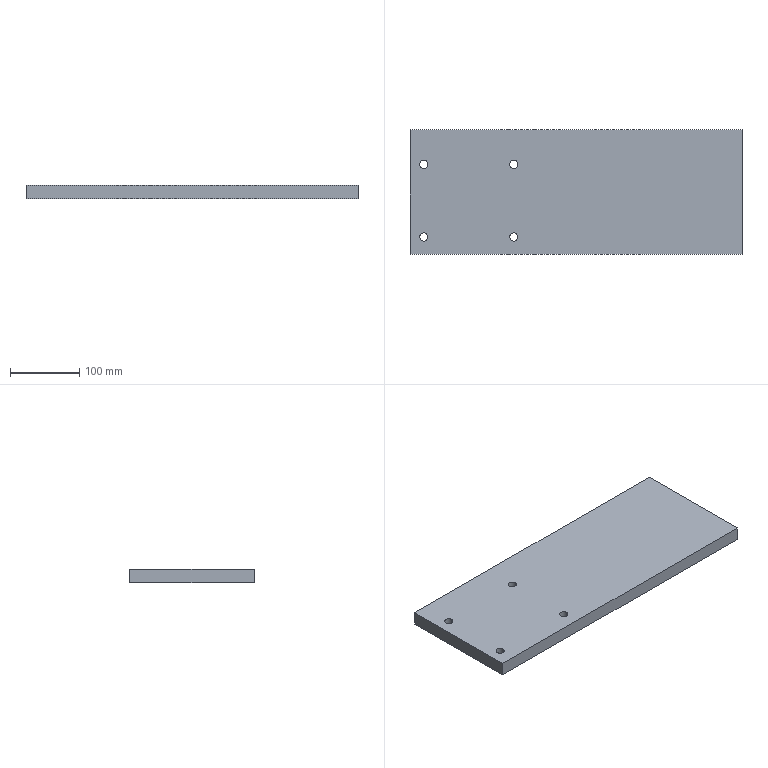Part | STEP file | Small Pad Plate | 1 solid | 14 faces | box 480 x 180 x 20 mm | volume 1718952 mm3 | cylinder 8 | plane 6 | commonest cylinder face diameters 12 x8
STEP:
#1=CARTESIAN_POINT('',(0.,0.,0.));
#2=DIRECTION('',(0.,0.,1.));
#3=DIRECTION('',(1.,0.,0.));
#4=AXIS2_PLACEMENT_3D('',#1,#2,#3);
#5=CARTESIAN_POINT('',(-84.,40.,0.));
#6=VERTEX_POINT('',#5);
#7=CARTESIAN_POINT('',(-84.,40.,20.));
#8=VERTEX_POINT('',#7);
#9=CARTESIAN_POINT('',(-84.,40.,20.));
#10=DIRECTION('',(0.,0.,1.));
#11=VECTOR('',#10,1.);
#12=LINE('',#9,#11);
#13=CARTESIAN_POINT('',(-90.,40.,20.));
#14=DIRECTION('',(0.,0.,1.));
#15=DIRECTION('',(1.,0.,0.));
#16=AXIS2_PLACEMENT_3D('',#13,#14,#15);
#17=CYLINDRICAL_SURFACE('',#16,6.);
#18=CARTESIAN_POINT('',(6.283,0.));
#19=DIRECTION('',(0.,1.));
#20=VECTOR('',#19,1.);
#21=LINE('',#18,#20);
#22=(GEOMETRIC_REPRESENTATION_CONTEXT(2)PARAMETRIC_REPRESENTATION_CONTEXT()REPRESENTATION_CONTEXT('',''));
#23=DEFINITIONAL_REPRESENTATION('',(#21),#22);
#24=PCURVE('',#17,#23);
#25=CARTESIAN_POINT('',(-90.,40.,20.));
#26=DIRECTION('',(0.,0.,1.));
#27=DIRECTION('',(1.,0.,0.));
#28=AXIS2_PLACEMENT_3D('',#25,#26,#27);
#29=CYLINDRICAL_SURFACE('',#28,6.);
#30=CARTESIAN_POINT('',(0.,0.));
#31=DIRECTION('',(0.,1.));
#32=VECTOR('',#31,1.);
#33=LINE('',#30,#32);
#34=(GEOMETRIC_REPRESENTATION_CONTEXT(2)PARAMETRIC_REPRESENTATION_CONTEXT()REPRESENTATION_CONTEXT('',''));
#35=DEFINITIONAL_REPRESENTATION('',(#33),#34);
#36=PCURVE('',#29,#35);
#37=SURFACE_CURVE('',#12,(#24,#36),.PCURVE_S1.);
#38=EDGE_CURVE('',#6,#8,#37,.T.);
#39=ORIENTED_EDGE('',*,*,#38,.T.);
#40=CARTESIAN_POINT('',(-96.,40.,20.));
#41=VERTEX_POINT('',#40);
#42=CARTESIAN_POINT('',(-90.,40.,20.));
#43=DIRECTION('',(0.,0.,1.));
#44=DIRECTION('',(1.,0.,0.));
#45=AXIS2_PLACEMENT_3D('',#42,#43,#44);
#46=CIRCLE('',#45,6.);
#47=CARTESIAN_POINT('',(0.,0.));
#48=DIRECTION('',(1.,0.));
#49=VECTOR('',#48,1.);
#50=LINE('',#47,#49);
#51=(GEOMETRIC_REPRESENTATION_CONTEXT(2)PARAMETRIC_REPRESENTATION_CONTEXT()REPRESENTATION_CONTEXT('',''));
#52=DEFINITIONAL_REPRESENTATION('',(#50),#51);
#53=PCURVE('',#17,#52);
#54=CARTESIAN_POINT('',(0.,0.,20.));
#55=DIRECTION('',(0.,0.,1.));
#56=DIRECTION('',(1.,0.,0.));
#57=AXIS2_PLACEMENT_3D('',#54,#55,#56);
#58=PLANE('',#57);
#59=CARTESIAN_POINT('',(-90.,40.));
#60=DIRECTION('',(1.,0.));
#61=AXIS2_PLACEMENT_2D('',#59,#60);
#62=CIRCLE('',#61,6.);
#63=(GEOMETRIC_REPRESENTATION_CONTEXT(2)PARAMETRIC_REPRESENTATION_CONTEXT()REPRESENTATION_CONTEXT('',''));
#64=DEFINITIONAL_REPRESENTATION('',(#62),#63);
#65=PCURVE('',#58,#64);
#66=SURFACE_CURVE('',#46,(#53,#65),.PCURVE_S1.);
#67=EDGE_CURVE('',#41,#8,#66,.T.);
#68=ORIENTED_EDGE('',*,*,#67,.F.);
#69=CARTESIAN_POINT('',(-96.,40.,0.));
#70=VERTEX_POINT('',#69);
#71=CARTESIAN_POINT('',(-96.,40.,20.));
#72=DIRECTION('',(0.,0.,1.));
#73=VECTOR('',#72,1.);
#74=LINE('',#71,#73);
#75=CARTESIAN_POINT('',(3.142,0.));
#76=DIRECTION('',(0.,1.));
#77=VECTOR('',#76,1.);
#78=LINE('',#75,#77);
#79=(GEOMETRIC_REPRESENTATION_CONTEXT(2)PARAMETRIC_REPRESENTATION_CONTEXT()REPRESENTATION_CONTEXT('',''));
#80=DEFINITIONAL_REPRESENTATION('',(#78),#79);
#81=PCURVE('',#17,#80);
#82=CARTESIAN_POINT('',(3.142,0.));
#83=DIRECTION('',(0.,1.));
#84=VECTOR('',#83,1.);
#85=LINE('',#82,#84);
#86=(GEOMETRIC_REPRESENTATION_CONTEXT(2)PARAMETRIC_REPRESENTATION_CONTEXT()REPRESENTATION_CONTEXT('',''));
#87=DEFINITIONAL_REPRESENTATION('',(#85),#86);
#88=PCURVE('',#29,#87);
#89=SURFACE_CURVE('',#74,(#81,#88),.PCURVE_S1.);
#90=EDGE_CURVE('',#70,#41,#89,.T.);
#91=ORIENTED_EDGE('',*,*,#90,.F.);
#92=CARTESIAN_POINT('',(-90.,40.,0.));
#93=DIRECTION('',(0.,0.,1.));
#94=DIRECTION('',(1.,0.,0.));
#95=AXIS2_PLACEMENT_3D('',#92,#93,#94);
#96=CIRCLE('',#95,6.);
#97=CARTESIAN_POINT('',(0.,-20.));
#98=DIRECTION('',(1.,0.));
#99=VECTOR('',#98,1.);
#100=LINE('',#97,#99);
#101=(GEOMETRIC_REPRESENTATION_CONTEXT(2)PARAMETRIC_REPRESENTATION_CONTEXT()REPRESENTATION_CONTEXT('',''));
#102=DEFINITIONAL_REPRESENTATION('',(#100),#101);
#103=PCURVE('',#17,#102);
#104=CARTESIAN_POINT('',(0.,0.,0.));
#105=DIRECTION('',(0.,0.,1.));
#106=DIRECTION('',(1.,0.,0.));
#107=AXIS2_PLACEMENT_3D('',#104,#105,#106);
#108=PLANE('',#107);
#109=CARTESIAN_POINT('',(-90.,40.));
#110=DIRECTION('',(1.,0.));
#111=AXIS2_PLACEMENT_2D('',#109,#110);
#112=CIRCLE('',#111,6.);
#113=(GEOMETRIC_REPRESENTATION_CONTEXT(2)PARAMETRIC_REPRESENTATION_CONTEXT()REPRESENTATION_CONTEXT('',''));
#114=DEFINITIONAL_REPRESENTATION('',(#112),#113);
#115=PCURVE('',#108,#114);
#116=SURFACE_CURVE('',#96,(#103,#115),.PCURVE_S1.);
#117=EDGE_CURVE('',#70,#6,#116,.T.);
#118=ORIENTED_EDGE('',*,*,#117,.T.);
#119=EDGE_LOOP('',(#39,#68,#91,#118));
#120=FACE_BOUND('',#119,.F.);
#121=ADVANCED_FACE('',(#120),#17,.F.);
#122=CARTESIAN_POINT('',(-84.,-65.,0.));
#123=VERTEX_POINT('',#122);
#124=CARTESIAN_POINT('',(-84.,-65.,20.));
#125=VERTEX_POINT('',#124);
#126=CARTESIAN_POINT('',(-84.,-65.,20.));
#127=DIRECTION('',(0.,0.,1.));
#128=VECTOR('',#127,1.);
#129=LINE('',#126,#128);
#130=CARTESIAN_POINT('',(-90.,-65.,20.));
#131=DIRECTION('',(0.,0.,1.));
#132=DIRECTION('',(1.,0.,0.));
#133=AXIS2_PLACEMENT_3D('',#130,#131,#132);
#134=CYLINDRICAL_SURFACE('',#133,6.);
#135=CARTESIAN_POINT('',(6.283,0.));
#136=DIRECTION('',(0.,1.));
#137=VECTOR('',#136,1.);
#138=LINE('',#135,#137);
#139=(GEOMETRIC_REPRESENTATION_CONTEXT(2)PARAMETRIC_REPRESENTATION_CONTEXT()REPRESENTATION_CONTEXT('',''));
#140=DEFINITIONAL_REPRESENTATION('',(#138),#139);
#141=PCURVE('',#134,#140);
#142=CARTESIAN_POINT('',(-90.,-65.,20.));
#143=DIRECTION('',(0.,0.,1.));
#144=DIRECTION('',(1.,0.,0.));
#145=AXIS2_PLACEMENT_3D('',#142,#143,#144);
#146=CYLINDRICAL_SURFACE('',#145,6.);
#147=CARTESIAN_POINT('',(0.,0.));
#148=DIRECTION('',(0.,1.));
#149=VECTOR('',#148,1.);
#150=LINE('',#147,#149);
#151=(GEOMETRIC_REPRESENTATION_CONTEXT(2)PARAMETRIC_REPRESENTATION_CONTEXT()REPRESENTATION_CONTEXT('',''));
#152=DEFINITIONAL_REPRESENTATION('',(#150),#151);
#153=PCURVE('',#146,#152);
#154=SURFACE_CURVE('',#129,(#141,#153),.PCURVE_S1.);
#155=EDGE_CURVE('',#123,#125,#154,.T.);
#156=ORIENTED_EDGE('',*,*,#155,.T.);
#157=CARTESIAN_POINT('',(-96.,-65.,20.));
#158=VERTEX_POINT('',#157);
#159=CARTESIAN_POINT('',(-90.,-65.,20.));
#160=DIRECTION('',(0.,0.,1.));
#161=DIRECTION('',(1.,0.,0.));
#162=AXIS2_PLACEMENT_3D('',#159,#160,#161);
#163=CIRCLE('',#162,6.);
#164=CARTESIAN_POINT('',(0.,0.));
#165=DIRECTION('',(1.,0.));
#166=VECTOR('',#165,1.);
#167=LINE('',#164,#166);
#168=(GEOMETRIC_REPRESENTATION_CONTEXT(2)PARAMETRIC_REPRESENTATION_CONTEXT()REPRESENTATION_CONTEXT('',''));
#169=DEFINITIONAL_REPRESENTATION('',(#167),#168);
#170=PCURVE('',#134,#169);
#171=CARTESIAN_POINT('',(-90.,-65.));
#172=DIRECTION('',(1.,0.));
#173=AXIS2_PLACEMENT_2D('',#171,#172);
#174=CIRCLE('',#173,6.);
#175=(GEOMETRIC_REPRESENTATION_CONTEXT(2)PARAMETRIC_REPRESENTATION_CONTEXT()REPRESENTATION_CONTEXT('',''));
#176=DEFINITIONAL_REPRESENTATION('',(#174),#175);
#177=PCURVE('',#58,#176);
#178=SURFACE_CURVE('',#163,(#170,#177),.PCURVE_S1.);
#179=EDGE_CURVE('',#158,#125,#178,.T.);
#180=ORIENTED_EDGE('',*,*,#179,.F.);
#181=CARTESIAN_POINT('',(-96.,-65.,0.));
#182=VERTEX_POINT('',#181);
#183=CARTESIAN_POINT('',(-96.,-65.,20.));
#184=DIRECTION('',(0.,0.,1.));
#185=VECTOR('',#184,1.);
#186=LINE('',#183,#185);
#187=CARTESIAN_POINT('',(3.142,0.));
#188=DIRECTION('',(0.,1.));
#189=VECTOR('',#188,1.);
#190=LINE('',#187,#189);
#191=(GEOMETRIC_REPRESENTATION_CONTEXT(2)PARAMETRIC_REPRESENTATION_CONTEXT()REPRESENTATION_CONTEXT('',''));
#192=DEFINITIONAL_REPRESENTATION('',(#190),#191);
#193=PCURVE('',#134,#192);
#194=CARTESIAN_POINT('',(3.142,0.));
#195=DIRECTION('',(0.,1.));
#196=VECTOR('',#195,1.);
#197=LINE('',#194,#196);
#198=(GEOMETRIC_REPRESENTATION_CONTEXT(2)PARAMETRIC_REPRESENTATION_CONTEXT()REPRESENTATION_CONTEXT('',''));
#199=DEFINITIONAL_REPRESENTATION('',(#197),#198);
#200=PCURVE('',#146,#199);
#201=SURFACE_CURVE('',#186,(#193,#200),.PCURVE_S1.);
#202=EDGE_CURVE('',#182,#158,#201,.T.);
#203=ORIENTED_EDGE('',*,*,#202,.F.);
#204=CARTESIAN_POINT('',(-90.,-65.,0.));
#205=DIRECTION('',(0.,0.,1.));
#206=DIRECTION('',(1.,0.,0.));
#207=AXIS2_PLACEMENT_3D('',#204,#205,#206);
#208=CIRCLE('',#207,6.);
#209=CARTESIAN_POINT('',(0.,-20.));
#210=DIRECTION('',(1.,0.));
#211=VECTOR('',#210,1.);
#212=LINE('',#209,#211);
#213=(GEOMETRIC_REPRESENTATION_CONTEXT(2)PARAMETRIC_REPRESENTATION_CONTEXT()REPRESENTATION_CONTEXT('',''));
#214=DEFINITIONAL_REPRESENTATION('',(#212),#213);
#215=PCURVE('',#134,#214);
#216=CARTESIAN_POINT('',(-90.,-65.));
#217=DIRECTION('',(1.,0.));
#218=AXIS2_PLACEMENT_2D('',#216,#217);
#219=CIRCLE('',#218,6.);
#220=(GEOMETRIC_REPRESENTATION_CONTEXT(2)PARAMETRIC_REPRESENTATION_CONTEXT()REPRESENTATION_CONTEXT('',''));
#221=DEFINITIONAL_REPRESENTATION('',(#219),#220);
#222=PCURVE('',#108,#221);
#223=SURFACE_CURVE('',#208,(#215,#222),.PCURVE_S1.);
#224=EDGE_CURVE('',#182,#123,#223,.T.);
#225=ORIENTED_EDGE('',*,*,#224,.T.);
#226=EDGE_LOOP('',(#156,#180,#203,#225));
#227=FACE_BOUND('',#226,.F.);
#228=ADVANCED_FACE('',(#227),#134,.F.);
#229=CARTESIAN_POINT('',(-214.,40.,0.));
#230=VERTEX_POINT('',#229);
#231=CARTESIAN_POINT('',(-214.,40.,20.));
#232=VERTEX_POINT('',#231);
#233=CARTESIAN_POINT('',(-214.,40.,20.));
#234=DIRECTION('',(0.,0.,1.));
#235=VECTOR('',#234,1.);
#236=LINE('',#233,#235);
#237=CARTESIAN_POINT('',(-220.,40.,20.));
#238=DIRECTION('',(0.,0.,1.));
#239=DIRECTION('',(1.,0.,0.));
#240=AXIS2_PLACEMENT_3D('',#237,#238,#239);
#241=CYLINDRICAL_SURFACE('',#240,6.);
#242=CARTESIAN_POINT('',(6.283,0.));
#243=DIRECTION('',(0.,1.));
#244=VECTOR('',#243,1.);
#245=LINE('',#242,#244);
#246=(GEOMETRIC_REPRESENTATION_CONTEXT(2)PARAMETRIC_REPRESENTATION_CONTEXT()REPRESENTATION_CONTEXT('',''));
#247=DEFINITIONAL_REPRESENTATION('',(#245),#246);
#248=PCURVE('',#241,#247);
#249=CARTESIAN_POINT('',(-220.,40.,20.));
#250=DIRECTION('',(0.,0.,1.));
#251=DIRECTION('',(1.,0.,0.));
#252=AXIS2_PLACEMENT_3D('',#249,#250,#251);
#253=CYLINDRICAL_SURFACE('',#252,6.);
#254=CARTESIAN_POINT('',(0.,0.));
#255=DIRECTION('',(0.,1.));
#256=VECTOR('',#255,1.);
#257=LINE('',#254,#256);
#258=(GEOMETRIC_REPRESENTATION_CONTEXT(2)PARAMETRIC_REPRESENTATION_CONTEXT()REPRESENTATION_CONTEXT('',''));
#259=DEFINITIONAL_REPRESENTATION('',(#257),#258);
#260=PCURVE('',#253,#259);
#261=SURFACE_CURVE('',#236,(#248,#260),.PCURVE_S1.);
#262=EDGE_CURVE('',#230,#232,#261,.T.);
#263=ORIENTED_EDGE('',*,*,#262,.T.);
#264=CARTESIAN_POINT('',(-226.,40.,20.));
#265=VERTEX_POINT('',#264);
#266=CARTESIAN_POINT('',(-220.,40.,20.));
#267=DIRECTION('',(0.,0.,1.));
#268=DIRECTION('',(1.,0.,0.));
#269=AXIS2_PLACEMENT_3D('',#266,#267,#268);
#270=CIRCLE('',#269,6.);
#271=CARTESIAN_POINT('',(0.,0.));
#272=DIRECTION('',(1.,0.));
#273=VECTOR('',#272,1.);
#274=LINE('',#271,#273);
#275=(GEOMETRIC_REPRESENTATION_CONTEXT(2)PARAMETRIC_REPRESENTATION_CONTEXT()REPRESENTATION_CONTEXT('',''));
#276=DEFINITIONAL_REPRESENTATION('',(#274),#275);
#277=PCURVE('',#241,#276);
#278=CARTESIAN_POINT('',(-220.,40.));
#279=DIRECTION('',(1.,0.));
#280=AXIS2_PLACEMENT_2D('',#278,#279);
#281=CIRCLE('',#280,6.);
#282=(GEOMETRIC_REPRESENTATION_CONTEXT(2)PARAMETRIC_REPRESENTATION_CONTEXT()REPRESENTATION_CONTEXT('',''));
#283=DEFINITIONAL_REPRESENTATION('',(#281),#282);
#284=PCURVE('',#58,#283);
#285=SURFACE_CURVE('',#270,(#277,#284),.PCURVE_S1.);
#286=EDGE_CURVE('',#265,#232,#285,.T.);
#287=ORIENTED_EDGE('',*,*,#286,.F.);
#288=CARTESIAN_POINT('',(-226.,40.,0.));
#289=VERTEX_POINT('',#288);
#290=CARTESIAN_POINT('',(-226.,40.,20.));
#291=DIRECTION('',(0.,0.,1.));
#292=VECTOR('',#291,1.);
#293=LINE('',#290,#292);
#294=CARTESIAN_POINT('',(3.142,0.));
#295=DIRECTION('',(0.,1.));
#296=VECTOR('',#295,1.);
#297=LINE('',#294,#296);
#298=(GEOMETRIC_REPRESENTATION_CONTEXT(2)PARAMETRIC_REPRESENTATION_CONTEXT()REPRESENTATION_CONTEXT('',''));
#299=DEFINITIONAL_REPRESENTATION('',(#297),#298);
#300=PCURVE('',#241,#299);
#301=CARTESIAN_POINT('',(3.142,0.));
#302=DIRECTION('',(0.,1.));
#303=VECTOR('',#302,1.);
#304=LINE('',#301,#303);
#305=(GEOMETRIC_REPRESENTATION_CONTEXT(2)PARAMETRIC_REPRESENTATION_CONTEXT()REPRESENTATION_CONTEXT('',''));
#306=DEFINITIONAL_REPRESENTATION('',(#304),#305);
#307=PCURVE('',#253,#306);
#308=SURFACE_CURVE('',#293,(#300,#307),.PCURVE_S1.);
#309=EDGE_CURVE('',#289,#265,#308,.T.);
#310=ORIENTED_EDGE('',*,*,#309,.F.);
#311=CARTESIAN_POINT('',(-220.,40.,0.));
#312=DIRECTION('',(0.,0.,1.));
#313=DIRECTION('',(1.,0.,0.));
#314=AXIS2_PLACEMENT_3D('',#311,#312,#313);
#315=CIRCLE('',#314,6.);
#316=CARTESIAN_POINT('',(0.,-20.));
#317=DIRECTION('',(1.,0.));
#318=VECTOR('',#317,1.);
#319=LINE('',#316,#318);
#320=(GEOMETRIC_REPRESENTATION_CONTEXT(2)PARAMETRIC_REPRESENTATION_CONTEXT()REPRESENTATION_CONTEXT('',''));
#321=DEFINITIONAL_REPRESENTATION('',(#319),#320);
#322=PCURVE('',#241,#321);
#323=CARTESIAN_POINT('',(-220.,40.));
#324=DIRECTION('',(1.,0.));
#325=AXIS2_PLACEMENT_2D('',#323,#324);
#326=CIRCLE('',#325,6.);
#327=(GEOMETRIC_REPRESENTATION_CONTEXT(2)PARAMETRIC_REPRESENTATION_CONTEXT()REPRESENTATION_CONTEXT('',''));
#328=DEFINITIONAL_REPRESENTATION('',(#326),#327);
#329=PCURVE('',#108,#328);
#330=SURFACE_CURVE('',#315,(#322,#329),.PCURVE_S1.);
#331=EDGE_CURVE('',#289,#230,#330,.T.);
#332=ORIENTED_EDGE('',*,*,#331,.T.);
#333=EDGE_LOOP('',(#263,#287,#310,#332));
#334=FACE_BOUND('',#333,.F.);
#335=ADVANCED_FACE('',(#334),#241,.F.);
#336=CARTESIAN_POINT('',(-214.,-65.,0.));
#337=VERTEX_POINT('',#336);
#338=CARTESIAN_POINT('',(-214.,-65.,20.));
#339=VERTEX_POINT('',#338);
#340=CARTESIAN_POINT('',(-214.,-65.,20.));
#341=DIRECTION('',(0.,0.,1.));
#342=VECTOR('',#341,1.);
#343=LINE('',#340,#342);
#344=CARTESIAN_POINT('',(-220.,-65.,20.));
#345=DIRECTION('',(0.,0.,1.));
#346=DIRECTION('',(1.,0.,0.));
#347=AXIS2_PLACEMENT_3D('',#344,#345,#346);
#348=CYLINDRICAL_SURFACE('',#347,6.);
#349=CARTESIAN_POINT('',(6.283,0.));
#350=DIRECTION('',(0.,1.));
#351=VECTOR('',#350,1.);
#352=LINE('',#349,#351);
#353=(GEOMETRIC_REPRESENTATION_CONTEXT(2)PARAMETRIC_REPRESENTATION_CONTEXT()REPRESENTATION_CONTEXT('',''));
#354=DEFINITIONAL_REPRESENTATION('',(#352),#353);
#355=PCURVE('',#348,#354);
#356=CARTESIAN_POINT('',(-220.,-65.,20.));
#357=DIRECTION('',(0.,0.,1.));
#358=DIRECTION('',(1.,0.,0.));
#359=AXIS2_PLACEMENT_3D('',#356,#357,#358);
#360=CYLINDRICAL_SURFACE('',#359,6.);
#361=CARTESIAN_POINT('',(0.,0.));
#362=DIRECTION('',(0.,1.));
#363=VECTOR('',#362,1.);
#364=LINE('',#361,#363);
#365=(GEOMETRIC_REPRESENTATION_CONTEXT(2)PARAMETRIC_REPRESENTATION_CONTEXT()REPRESENTATION_CONTEXT('',''));
#366=DEFINITIONAL_REPRESENTATION('',(#364),#365);
#367=PCURVE('',#360,#366);
#368=SURFACE_CURVE('',#343,(#355,#367),.PCURVE_S1.);
#369=EDGE_CURVE('',#337,#339,#368,.T.);
#370=ORIENTED_EDGE('',*,*,#369,.T.);
#371=CARTESIAN_POINT('',(-226.,-65.,20.));
#372=VERTEX_POINT('',#371);
#373=CARTESIAN_POINT('',(-220.,-65.,20.));
#374=DIRECTION('',(0.,0.,1.));
#375=DIRECTION('',(1.,0.,0.));
#376=AXIS2_PLACEMENT_3D('',#373,#374,#375);
#377=CIRCLE('',#376,6.);
#378=CARTESIAN_POINT('',(0.,0.));
#379=DIRECTION('',(1.,0.));
#380=VECTOR('',#379,1.);
#381=LINE('',#378,#380);
#382=(GEOMETRIC_REPRESENTATION_CONTEXT(2)PARAMETRIC_REPRESENTATION_CONTEXT()REPRESENTATION_CONTEXT('',''));
#383=DEFINITIONAL_REPRESENTATION('',(#381),#382);
#384=PCURVE('',#348,#383);
#385=CARTESIAN_POINT('',(-220.,-65.));
#386=DIRECTION('',(1.,0.));
#387=AXIS2_PLACEMENT_2D('',#385,#386);
#388=CIRCLE('',#387,6.);
#389=(GEOMETRIC_REPRESENTATION_CONTEXT(2)PARAMETRIC_REPRESENTATION_CONTEXT()REPRESENTATION_CONTEXT('',''));
#390=DEFINITIONAL_REPRESENTATION('',(#388),#389);
#391=PCURVE('',#58,#390);
#392=SURFACE_CURVE('',#377,(#384,#391),.PCURVE_S1.);
#393=EDGE_CURVE('',#372,#339,#392,.T.);
#394=ORIENTED_EDGE('',*,*,#393,.F.);
#395=CARTESIAN_POINT('',(-226.,-65.,0.));
#396=VERTEX_POINT('',#395);
#397=CARTESIAN_POINT('',(-226.,-65.,20.));
#398=DIRECTION('',(0.,0.,1.));
#399=VECTOR('',#398,1.);
#400=LINE('',#397,#399);
#401=CARTESIAN_POINT('',(3.142,0.));
#402=DIRECTION('',(0.,1.));
#403=VECTOR('',#402,1.);
#404=LINE('',#401,#403);
#405=(GEOMETRIC_REPRESENTATION_CONTEXT(2)PARAMETRIC_REPRESENTATION_CONTEXT()REPRESENTATION_CONTEXT('',''));
#406=DEFINITIONAL_REPRESENTATION('',(#404),#405);
#407=PCURVE('',#348,#406);
#408=CARTESIAN_POINT('',(3.142,0.));
#409=DIRECTION('',(0.,1.));
#410=VECTOR('',#409,1.);
#411=LINE('',#408,#410);
#412=(GEOMETRIC_REPRESENTATION_CONTEXT(2)PARAMETRIC_REPRESENTATION_CONTEXT()REPRESENTATION_CONTEXT('',''));
#413=DEFINITIONAL_REPRESENTATION('',(#411),#412);
#414=PCURVE('',#360,#413);
#415=SURFACE_CURVE('',#400,(#407,#414),.PCURVE_S1.);
#416=EDGE_CURVE('',#396,#372,#415,.T.);
#417=ORIENTED_EDGE('',*,*,#416,.F.);
#418=CARTESIAN_POINT('',(-220.,-65.,0.));
#419=DIRECTION('',(0.,0.,1.));
#420=DIRECTION('',(1.,0.,0.));
#421=AXIS2_PLACEMENT_3D('',#418,#419,#420);
#422=CIRCLE('',#421,6.);
#423=CARTESIAN_POINT('',(0.,-20.));
#424=DIRECTION('',(1.,0.));
#425=VECTOR('',#424,1.);
#426=LINE('',#423,#425);
#427=(GEOMETRIC_REPRESENTATION_CONTEXT(2)PARAMETRIC_REPRESENTATION_CONTEXT()REPRESENTATION_CONTEXT('',''));
#428=DEFINITIONAL_REPRESENTATION('',(#426),#427);
#429=PCURVE('',#348,#428);
#430=CARTESIAN_POINT('',(-220.,-65.));
#431=DIRECTION('',(1.,0.));
#432=AXIS2_PLACEMENT_2D('',#430,#431);
#433=CIRCLE('',#432,6.);
#434=(GEOMETRIC_REPRESENTATION_CONTEXT(2)PARAMETRIC_REPRESENTATION_CONTEXT()REPRESENTATION_CONTEXT('',''));
#435=DEFINITIONAL_REPRESENTATION('',(#433),#434);
#436=PCURVE('',#108,#435);
#437=SURFACE_CURVE('',#422,(#429,#436),.PCURVE_S1.);
#438=EDGE_CURVE('',#396,#337,#437,.T.);
#439=ORIENTED_EDGE('',*,*,#438,.T.);
#440=EDGE_LOOP('',(#370,#394,#417,#439));
#441=FACE_BOUND('',#440,.F.);
#442=ADVANCED_FACE('',(#441),#348,.F.);
#443=CARTESIAN_POINT('',(240.,-90.,0.));
#444=VERTEX_POINT('',#443);
#445=CARTESIAN_POINT('',(240.,90.,0.));
#446=VERTEX_POINT('',#445);
#447=CARTESIAN_POINT('',(240.,90.,0.));
#448=DIRECTION('',(0.,1.,0.));
#449=VECTOR('',#448,1.);
#450=LINE('',#447,#449);
#451=CARTESIAN_POINT('',(240.,90.,20.));
#452=DIRECTION('',(-1.,0.,0.));
#453=DIRECTION('',(0.,-1.,0.));
#454=AXIS2_PLACEMENT_3D('',#451,#452,#453);
#455=PLANE('',#454);
#456=CARTESIAN_POINT('',(0.,-20.));
#457=DIRECTION('',(-1.,0.));
#458=VECTOR('',#457,1.);
#459=LINE('',#456,#458);
#460=(GEOMETRIC_REPRESENTATION_CONTEXT(2)PARAMETRIC_REPRESENTATION_CONTEXT()REPRESENTATION_CONTEXT('',''));
#461=DEFINITIONAL_REPRESENTATION('',(#459),#460);
#462=PCURVE('',#455,#461);
#463=CARTESIAN_POINT('',(240.,90.));
#464=DIRECTION('',(0.,1.));
#465=VECTOR('',#464,1.);
#466=LINE('',#463,#465);
#467=(GEOMETRIC_REPRESENTATION_CONTEXT(2)PARAMETRIC_REPRESENTATION_CONTEXT()REPRESENTATION_CONTEXT('',''));
#468=DEFINITIONAL_REPRESENTATION('',(#466),#467);
#469=PCURVE('',#108,#468);
#470=SURFACE_CURVE('',#450,(#462,#469),.PCURVE_S1.);
#471=EDGE_CURVE('',#444,#446,#470,.T.);
#472=ORIENTED_EDGE('',*,*,#471,.T.);
#473=CARTESIAN_POINT('',(240.,90.,20.));
#474=VERTEX_POINT('',#473);
#475=CARTESIAN_POINT('',(240.,90.,20.));
#476=DIRECTION('',(0.,0.,-1.));
#477=VECTOR('',#476,1.);
#478=LINE('',#475,#477);
#479=CARTESIAN_POINT('',(0.,0.));
#480=DIRECTION('',(0.,-1.));
#481=VECTOR('',#480,1.);
#482=LINE('',#479,#481);
#483=(GEOMETRIC_REPRESENTATION_CONTEXT(2)PARAMETRIC_REPRESENTATION_CONTEXT()REPRESENTATION_CONTEXT('',''));
#484=DEFINITIONAL_REPRESENTATION('',(#482),#483);
#485=PCURVE('',#455,#484);
#486=CARTESIAN_POINT('',(-240.,90.,20.));
#487=DIRECTION('',(0.,-1.,0.));
#488=DIRECTION('',(0.,0.,-1.));
#489=AXIS2_PLACEMENT_3D('',#486,#487,#488);
#490=PLANE('',#489);
#491=CARTESIAN_POINT('',(0.,480.));
#492=DIRECTION('',(1.,0.));
#493=VECTOR('',#492,1.);
#494=LINE('',#491,#493);
#495=(GEOMETRIC_REPRESENTATION_CONTEXT(2)PARAMETRIC_REPRESENTATION_CONTEXT()REPRESENTATION_CONTEXT('',''));
#496=DEFINITIONAL_REPRESENTATION('',(#494),#495);
#497=PCURVE('',#490,#496);
#498=SURFACE_CURVE('',#478,(#485,#497),.PCURVE_S1.);
#499=EDGE_CURVE('',#474,#446,#498,.T.);
#500=ORIENTED_EDGE('',*,*,#499,.F.);
#501=CARTESIAN_POINT('',(240.,-90.,20.));
#502=VERTEX_POINT('',#501);
#503=CARTESIAN_POINT('',(240.,90.,20.));
#504=DIRECTION('',(0.,1.,0.));
#505=VECTOR('',#504,1.);
#506=LINE('',#503,#505);
#507=CARTESIAN_POINT('',(0.,0.));
#508=DIRECTION('',(-1.,0.));
#509=VECTOR('',#508,1.);
#510=LINE('',#507,#509);
#511=(GEOMETRIC_REPRESENTATION_CONTEXT(2)PARAMETRIC_REPRESENTATION_CONTEXT()REPRESENTATION_CONTEXT('',''));
#512=DEFINITIONAL_REPRESENTATION('',(#510),#511);
#513=PCURVE('',#455,#512);
#514=CARTESIAN_POINT('',(240.,90.));
#515=DIRECTION('',(0.,1.));
#516=VECTOR('',#515,1.);
#517=LINE('',#514,#516);
#518=(GEOMETRIC_REPRESENTATION_CONTEXT(2)PARAMETRIC_REPRESENTATION_CONTEXT()REPRESENTATION_CONTEXT('',''));
#519=DEFINITIONAL_REPRESENTATION('',(#517),#518);
#520=PCURVE('',#58,#519);
#521=SURFACE_CURVE('',#506,(#513,#520),.PCURVE_S1.);
#522=EDGE_CURVE('',#502,#474,#521,.T.);
#523=ORIENTED_EDGE('',*,*,#522,.F.);
#524=CARTESIAN_POINT('',(240.,-90.,20.));
#525=DIRECTION('',(0.,0.,-1.));
#526=VECTOR('',#525,1.);
#527=LINE('',#524,#526);
#528=CARTESIAN_POINT('',(180.,0.));
#529=DIRECTION('',(0.,-1.));
#530=VECTOR('',#529,1.);
#531=LINE('',#528,#530);
#532=(GEOMETRIC_REPRESENTATION_CONTEXT(2)PARAMETRIC_REPRESENTATION_CONTEXT()REPRESENTATION_CONTEXT('',''));
#533=DEFINITIONAL_REPRESENTATION('',(#531),#532);
#534=PCURVE('',#455,#533);
#535=CARTESIAN_POINT('',(-240.,-90.,20.));
#536=DIRECTION('',(0.,1.,0.));
#537=DIRECTION('',(0.,0.,1.));
#538=AXIS2_PLACEMENT_3D('',#535,#536,#537);
#539=PLANE('',#538);
#540=CARTESIAN_POINT('',(0.,480.));
#541=DIRECTION('',(-1.,0.));
#542=VECTOR('',#541,1.);
#543=LINE('',#540,#542);
#544=(GEOMETRIC_REPRESENTATION_CONTEXT(2)PARAMETRIC_REPRESENTATION_CONTEXT()REPRESENTATION_CONTEXT('',''));
#545=DEFINITIONAL_REPRESENTATION('',(#543),#544);
#546=PCURVE('',#539,#545);
#547=SURFACE_CURVE('',#527,(#534,#546),.PCURVE_S1.);
#548=EDGE_CURVE('',#502,#444,#547,.T.);
#549=ORIENTED_EDGE('',*,*,#548,.T.);
#550=EDGE_LOOP('',(#472,#500,#523,#549));
#551=FACE_BOUND('',#550,.T.);
#552=ADVANCED_FACE('',(#551),#455,.F.);
#553=CARTESIAN_POINT('',(-240.,90.,0.));
#554=VERTEX_POINT('',#553);
#555=CARTESIAN_POINT('',(-240.,90.,0.));
#556=DIRECTION('',(-1.,0.,0.));
#557=VECTOR('',#556,1.);
#558=LINE('',#555,#557);
#559=CARTESIAN_POINT('',(20.,0.));
#560=DIRECTION('',(0.,-1.));
#561=VECTOR('',#560,1.);
#562=LINE('',#559,#561);
#563=(GEOMETRIC_REPRESENTATION_CONTEXT(2)PARAMETRIC_REPRESENTATION_CONTEXT()REPRESENTATION_CONTEXT('',''));
#564=DEFINITIONAL_REPRESENTATION('',(#562),#563);
#565=PCURVE('',#490,#564);
#566=CARTESIAN_POINT('',(-240.,90.));
#567=DIRECTION('',(-1.,0.));
#568=VECTOR('',#567,1.);
#569=LINE('',#566,#568);
#570=(GEOMETRIC_REPRESENTATION_CONTEXT(2)PARAMETRIC_REPRESENTATION_CONTEXT()REPRESENTATION_CONTEXT('',''));
#571=DEFINITIONAL_REPRESENTATION('',(#569),#570);
#572=PCURVE('',#108,#571);
#573=SURFACE_CURVE('',#558,(#565,#572),.PCURVE_S1.);
#574=EDGE_CURVE('',#446,#554,#573,.T.);
#575=ORIENTED_EDGE('',*,*,#574,.T.);
#576=CARTESIAN_POINT('',(-240.,90.,20.));
#577=VERTEX_POINT('',#576);
#578=CARTESIAN_POINT('',(-240.,90.,20.));
#579=DIRECTION('',(0.,0.,-1.));
#580=VECTOR('',#579,1.);
#581=LINE('',#578,#580);
#582=CARTESIAN_POINT('',(0.,0.));
#583=DIRECTION('',(1.,0.));
#584=VECTOR('',#583,1.);
#585=LINE('',#582,#584);
#586=(GEOMETRIC_REPRESENTATION_CONTEXT(2)PARAMETRIC_REPRESENTATION_CONTEXT()REPRESENTATION_CONTEXT('',''));
#587=DEFINITIONAL_REPRESENTATION('',(#585),#586);
#588=PCURVE('',#490,#587);
#589=CARTESIAN_POINT('',(-240.,90.,20.));
#590=DIRECTION('',(1.,0.,0.));
#591=DIRECTION('',(0.,1.,0.));
#592=AXIS2_PLACEMENT_3D('',#589,#590,#591);
#593=PLANE('',#592);
#594=CARTESIAN_POINT('',(0.,0.));
#595=DIRECTION('',(0.,-1.));
#596=VECTOR('',#595,1.);
#597=LINE('',#594,#596);
#598=(GEOMETRIC_REPRESENTATION_CONTEXT(2)PARAMETRIC_REPRESENTATION_CONTEXT()REPRESENTATION_CONTEXT('',''));
#599=DEFINITIONAL_REPRESENTATION('',(#597),#598);
#600=PCURVE('',#593,#599);
#601=SURFACE_CURVE('',#581,(#588,#600),.PCURVE_S1.);
#602=EDGE_CURVE('',#577,#554,#601,.T.);
#603=ORIENTED_EDGE('',*,*,#602,.F.);
#604=CARTESIAN_POINT('',(-240.,90.,20.));
#605=DIRECTION('',(-1.,0.,0.));
#606=VECTOR('',#605,1.);
#607=LINE('',#604,#606);
#608=CARTESIAN_POINT('',(0.,0.));
#609=DIRECTION('',(0.,-1.));
#610=VECTOR('',#609,1.);
#611=LINE('',#608,#610);
#612=(GEOMETRIC_REPRESENTATION_CONTEXT(2)PARAMETRIC_REPRESENTATION_CONTEXT()REPRESENTATION_CONTEXT('',''));
#613=DEFINITIONAL_REPRESENTATION('',(#611),#612);
#614=PCURVE('',#490,#613);
#615=CARTESIAN_POINT('',(-240.,90.));
#616=DIRECTION('',(-1.,0.));
#617=VECTOR('',#616,1.);
#618=LINE('',#615,#617);
#619=(GEOMETRIC_REPRESENTATION_CONTEXT(2)PARAMETRIC_REPRESENTATION_CONTEXT()REPRESENTATION_CONTEXT('',''));
#620=DEFINITIONAL_REPRESENTATION('',(#618),#619);
#621=PCURVE('',#58,#620);
#622=SURFACE_CURVE('',#607,(#614,#621),.PCURVE_S1.);
#623=EDGE_CURVE('',#474,#577,#622,.T.);
#624=ORIENTED_EDGE('',*,*,#623,.F.);
#625=ORIENTED_EDGE('',*,*,#499,.T.);
#626=EDGE_LOOP('',(#575,#603,#624,#625));
#627=FACE_BOUND('',#626,.T.);
#628=ADVANCED_FACE('',(#627),#490,.F.);
#629=CARTESIAN_POINT('',(-240.,-90.,0.));
#630=VERTEX_POINT('',#629);
#631=CARTESIAN_POINT('',(-240.,90.,0.));
#632=DIRECTION('',(0.,-1.,0.));
#633=VECTOR('',#632,1.);
#634=LINE('',#631,#633);
#635=CARTESIAN_POINT('',(0.,-20.));
#636=DIRECTION('',(-1.,0.));
#637=VECTOR('',#636,1.);
#638=LINE('',#635,#637);
#639=(GEOMETRIC_REPRESENTATION_CONTEXT(2)PARAMETRIC_REPRESENTATION_CONTEXT()REPRESENTATION_CONTEXT('',''));
#640=DEFINITIONAL_REPRESENTATION('',(#638),#639);
#641=PCURVE('',#593,#640);
#642=CARTESIAN_POINT('',(-240.,90.));
#643=DIRECTION('',(0.,-1.));
#644=VECTOR('',#643,1.);
#645=LINE('',#642,#644);
#646=(GEOMETRIC_REPRESENTATION_CONTEXT(2)PARAMETRIC_REPRESENTATION_CONTEXT()REPRESENTATION_CONTEXT('',''));
#647=DEFINITIONAL_REPRESENTATION('',(#645),#646);
#648=PCURVE('',#108,#647);
#649=SURFACE_CURVE('',#634,(#641,#648),.PCURVE_S1.);
#650=EDGE_CURVE('',#554,#630,#649,.T.);
#651=ORIENTED_EDGE('',*,*,#650,.T.);
#652=CARTESIAN_POINT('',(-240.,-90.,20.));
#653=VERTEX_POINT('',#652);
#654=CARTESIAN_POINT('',(-240.,-90.,20.));
#655=DIRECTION('',(0.,0.,-1.));
#656=VECTOR('',#655,1.);
#657=LINE('',#654,#656);
#658=CARTESIAN_POINT('',(-180.,0.));
#659=DIRECTION('',(0.,-1.));
#660=VECTOR('',#659,1.);
#661=LINE('',#658,#660);
#662=(GEOMETRIC_REPRESENTATION_CONTEXT(2)PARAMETRIC_REPRESENTATION_CONTEXT()REPRESENTATION_CONTEXT('',''));
#663=DEFINITIONAL_REPRESENTATION('',(#661),#662);
#664=PCURVE('',#593,#663);
#665=CARTESIAN_POINT('',(0.,0.));
#666=DIRECTION('',(-1.,0.));
#667=VECTOR('',#666,1.);
#668=LINE('',#665,#667);
#669=(GEOMETRIC_REPRESENTATION_CONTEXT(2)PARAMETRIC_REPRESENTATION_CONTEXT()REPRESENTATION_CONTEXT('',''));
#670=DEFINITIONAL_REPRESENTATION('',(#668),#669);
#671=PCURVE('',#539,#670);
#672=SURFACE_CURVE('',#657,(#664,#671),.PCURVE_S1.);
#673=EDGE_CURVE('',#653,#630,#672,.T.);
#674=ORIENTED_EDGE('',*,*,#673,.F.);
#675=CARTESIAN_POINT('',(-240.,90.,20.));
#676=DIRECTION('',(0.,-1.,0.));
#677=VECTOR('',#676,1.);
#678=LINE('',#675,#677);
#679=CARTESIAN_POINT('',(0.,0.));
#680=DIRECTION('',(-1.,0.));
#681=VECTOR('',#680,1.);
#682=LINE('',#679,#681);
#683=(GEOMETRIC_REPRESENTATION_CONTEXT(2)PARAMETRIC_REPRESENTATION_CONTEXT()REPRESENTATION_CONTEXT('',''));
#684=DEFINITIONAL_REPRESENTATION('',(#682),#683);
#685=PCURVE('',#593,#684);
#686=CARTESIAN_POINT('',(-240.,90.));
#687=DIRECTION('',(0.,-1.));
#688=VECTOR('',#687,1.);
#689=LINE('',#686,#688);
#690=(GEOMETRIC_REPRESENTATION_CONTEXT(2)PARAMETRIC_REPRESENTATION_CONTEXT()REPRESENTATION_CONTEXT('',''));
#691=DEFINITIONAL_REPRESENTATION('',(#689),#690);
#692=PCURVE('',#58,#691);
#693=SURFACE_CURVE('',#678,(#685,#692),.PCURVE_S1.);
#694=EDGE_CURVE('',#577,#653,#693,.T.);
#695=ORIENTED_EDGE('',*,*,#694,.F.);
#696=ORIENTED_EDGE('',*,*,#602,.T.);
#697=EDGE_LOOP('',(#651,#674,#695,#696));
#698=FACE_BOUND('',#697,.T.);
#699=ADVANCED_FACE('',(#698),#593,.F.);
#700=CARTESIAN_POINT('',(-240.,-90.,0.));
#701=DIRECTION('',(1.,0.,0.));
#702=VECTOR('',#701,1.);
#703=LINE('',#700,#702);
#704=CARTESIAN_POINT('',(-20.,0.));
#705=DIRECTION('',(0.,1.));
#706=VECTOR('',#705,1.);
#707=LINE('',#704,#706);
#708=(GEOMETRIC_REPRESENTATION_CONTEXT(2)PARAMETRIC_REPRESENTATION_CONTEXT()REPRESENTATION_CONTEXT('',''));
#709=DEFINITIONAL_REPRESENTATION('',(#707),#708);
#710=PCURVE('',#539,#709);
#711=CARTESIAN_POINT('',(-240.,-90.));
#712=DIRECTION('',(1.,0.));
#713=VECTOR('',#712,1.);
#714=LINE('',#711,#713);
#715=(GEOMETRIC_REPRESENTATION_CONTEXT(2)PARAMETRIC_REPRESENTATION_CONTEXT()REPRESENTATION_CONTEXT('',''));
#716=DEFINITIONAL_REPRESENTATION('',(#714),#715);
#717=PCURVE('',#108,#716);
#718=SURFACE_CURVE('',#703,(#710,#717),.PCURVE_S1.);
#719=EDGE_CURVE('',#630,#444,#718,.T.);
#720=ORIENTED_EDGE('',*,*,#719,.T.);
#721=ORIENTED_EDGE('',*,*,#548,.F.);
#722=CARTESIAN_POINT('',(-240.,-90.,20.));
#723=DIRECTION('',(1.,0.,0.));
#724=VECTOR('',#723,1.);
#725=LINE('',#722,#724);
#726=CARTESIAN_POINT('',(0.,0.));
#727=DIRECTION('',(0.,1.));
#728=VECTOR('',#727,1.);
#729=LINE('',#726,#728);
#730=(GEOMETRIC_REPRESENTATION_CONTEXT(2)PARAMETRIC_REPRESENTATION_CONTEXT()REPRESENTATION_CONTEXT('',''));
#731=DEFINITIONAL_REPRESENTATION('',(#729),#730);
#732=PCURVE('',#539,#731);
#733=CARTESIAN_POINT('',(-240.,-90.));
#734=DIRECTION('',(1.,0.));
#735=VECTOR('',#734,1.);
#736=LINE('',#733,#735);
#737=(GEOMETRIC_REPRESENTATION_CONTEXT(2)PARAMETRIC_REPRESENTATION_CONTEXT()REPRESENTATION_CONTEXT('',''));
#738=DEFINITIONAL_REPRESENTATION('',(#736),#737);
#739=PCURVE('',#58,#738);
#740=SURFACE_CURVE('',#725,(#732,#739),.PCURVE_S1.);
#741=EDGE_CURVE('',#653,#502,#740,.T.);
#742=ORIENTED_EDGE('',*,*,#741,.F.);
#743=ORIENTED_EDGE('',*,*,#673,.T.);
#744=EDGE_LOOP('',(#720,#721,#742,#743));
#745=FACE_BOUND('',#744,.T.);
#746=ADVANCED_FACE('',(#745),#539,.F.);
#747=CARTESIAN_POINT('',(-90.,40.,20.));
#748=DIRECTION('',(0.,0.,1.));
#749=DIRECTION('',(1.,0.,0.));
#750=AXIS2_PLACEMENT_3D('',#747,#748,#749);
#751=CIRCLE('',#750,6.);
#752=CARTESIAN_POINT('',(-90.,40.));
#753=DIRECTION('',(1.,0.));
#754=AXIS2_PLACEMENT_2D('',#752,#753);
#755=CIRCLE('',#754,6.);
#756=(GEOMETRIC_REPRESENTATION_CONTEXT(2)PARAMETRIC_REPRESENTATION_CONTEXT()REPRESENTATION_CONTEXT('',''));
#757=DEFINITIONAL_REPRESENTATION('',(#755),#756);
#758=PCURVE('',#58,#757);
#759=CARTESIAN_POINT('',(0.,0.));
#760=DIRECTION('',(1.,0.));
#761=VECTOR('',#760,1.);
#762=LINE('',#759,#761);
#763=(GEOMETRIC_REPRESENTATION_CONTEXT(2)PARAMETRIC_REPRESENTATION_CONTEXT()REPRESENTATION_CONTEXT('',''));
#764=DEFINITIONAL_REPRESENTATION('',(#762),#763);
#765=PCURVE('',#29,#764);
#766=SURFACE_CURVE('',#751,(#758,#765),.PCURVE_S1.);
#767=EDGE_CURVE('',#8,#41,#766,.T.);
#768=ORIENTED_EDGE('',*,*,#767,.F.);
#769=ORIENTED_EDGE('',*,*,#67,.F.);
#770=EDGE_LOOP('',(#768,#769));
#771=FACE_BOUND('',#770,.T.);
#772=CARTESIAN_POINT('',(-90.,-65.,20.));
#773=DIRECTION('',(0.,0.,1.));
#774=DIRECTION('',(1.,0.,0.));
#775=AXIS2_PLACEMENT_3D('',#772,#773,#774);
#776=CIRCLE('',#775,6.);
#777=CARTESIAN_POINT('',(-90.,-65.));
#778=DIRECTION('',(1.,0.));
#779=AXIS2_PLACEMENT_2D('',#777,#778);
#780=CIRCLE('',#779,6.);
#781=(GEOMETRIC_REPRESENTATION_CONTEXT(2)PARAMETRIC_REPRESENTATION_CONTEXT()REPRESENTATION_CONTEXT('',''));
#782=DEFINITIONAL_REPRESENTATION('',(#780),#781);
#783=PCURVE('',#58,#782);
#784=CARTESIAN_POINT('',(0.,0.));
#785=DIRECTION('',(1.,0.));
#786=VECTOR('',#785,1.);
#787=LINE('',#784,#786);
#788=(GEOMETRIC_REPRESENTATION_CONTEXT(2)PARAMETRIC_REPRESENTATION_CONTEXT()REPRESENTATION_CONTEXT('',''));
#789=DEFINITIONAL_REPRESENTATION('',(#787),#788);
#790=PCURVE('',#146,#789);
#791=SURFACE_CURVE('',#776,(#783,#790),.PCURVE_S1.);
#792=EDGE_CURVE('',#125,#158,#791,.T.);
#793=ORIENTED_EDGE('',*,*,#792,.F.);
#794=ORIENTED_EDGE('',*,*,#179,.F.);
#795=EDGE_LOOP('',(#793,#794));
#796=FACE_BOUND('',#795,.T.);
#797=CARTESIAN_POINT('',(-220.,40.,20.));
#798=DIRECTION('',(0.,0.,1.));
#799=DIRECTION('',(1.,0.,0.));
#800=AXIS2_PLACEMENT_3D('',#797,#798,#799);
#801=CIRCLE('',#800,6.);
#802=CARTESIAN_POINT('',(-220.,40.));
#803=DIRECTION('',(1.,0.));
#804=AXIS2_PLACEMENT_2D('',#802,#803);
#805=CIRCLE('',#804,6.);
#806=(GEOMETRIC_REPRESENTATION_CONTEXT(2)PARAMETRIC_REPRESENTATION_CONTEXT()REPRESENTATION_CONTEXT('',''));
#807=DEFINITIONAL_REPRESENTATION('',(#805),#806);
#808=PCURVE('',#58,#807);
#809=CARTESIAN_POINT('',(0.,0.));
#810=DIRECTION('',(1.,0.));
#811=VECTOR('',#810,1.);
#812=LINE('',#809,#811);
#813=(GEOMETRIC_REPRESENTATION_CONTEXT(2)PARAMETRIC_REPRESENTATION_CONTEXT()REPRESENTATION_CONTEXT('',''));
#814=DEFINITIONAL_REPRESENTATION('',(#812),#813);
#815=PCURVE('',#253,#814);
#816=SURFACE_CURVE('',#801,(#808,#815),.PCURVE_S1.);
#817=EDGE_CURVE('',#232,#265,#816,.T.);
#818=ORIENTED_EDGE('',*,*,#817,.F.);
#819=ORIENTED_EDGE('',*,*,#286,.F.);
#820=EDGE_LOOP('',(#818,#819));
#821=FACE_BOUND('',#820,.T.);
#822=CARTESIAN_POINT('',(-220.,-65.,20.));
#823=DIRECTION('',(0.,0.,1.));
#824=DIRECTION('',(1.,0.,0.));
#825=AXIS2_PLACEMENT_3D('',#822,#823,#824);
#826=CIRCLE('',#825,6.);
#827=CARTESIAN_POINT('',(-220.,-65.));
#828=DIRECTION('',(1.,0.));
#829=AXIS2_PLACEMENT_2D('',#827,#828);
#830=CIRCLE('',#829,6.);
#831=(GEOMETRIC_REPRESENTATION_CONTEXT(2)PARAMETRIC_REPRESENTATION_CONTEXT()REPRESENTATION_CONTEXT('',''));
#832=DEFINITIONAL_REPRESENTATION('',(#830),#831);
#833=PCURVE('',#58,#832);
#834=CARTESIAN_POINT('',(0.,0.));
#835=DIRECTION('',(1.,0.));
#836=VECTOR('',#835,1.);
#837=LINE('',#834,#836);
#838=(GEOMETRIC_REPRESENTATION_CONTEXT(2)PARAMETRIC_REPRESENTATION_CONTEXT()REPRESENTATION_CONTEXT('',''));
#839=DEFINITIONAL_REPRESENTATION('',(#837),#838);
#840=PCURVE('',#360,#839);
#841=SURFACE_CURVE('',#826,(#833,#840),.PCURVE_S1.);
#842=EDGE_CURVE('',#339,#372,#841,.T.);
#843=ORIENTED_EDGE('',*,*,#842,.F.);
#844=ORIENTED_EDGE('',*,*,#393,.F.);
#845=EDGE_LOOP('',(#843,#844));
#846=FACE_BOUND('',#845,.T.);
#847=ORIENTED_EDGE('',*,*,#522,.T.);
#848=ORIENTED_EDGE('',*,*,#623,.T.);
#849=ORIENTED_EDGE('',*,*,#694,.T.);
#850=ORIENTED_EDGE('',*,*,#741,.T.);
#851=EDGE_LOOP('',(#847,#848,#849,#850));
#852=FACE_BOUND('',#851,.T.);
#853=ADVANCED_FACE('',(#771,#796,#821,#846,#852),#58,.T.);
#854=CARTESIAN_POINT('',(-90.,40.,0.));
#855=DIRECTION('',(0.,0.,1.));
#856=DIRECTION('',(1.,0.,0.));
#857=AXIS2_PLACEMENT_3D('',#854,#855,#856);
#858=CIRCLE('',#857,6.);
#859=CARTESIAN_POINT('',(-90.,40.));
#860=DIRECTION('',(1.,0.));
#861=AXIS2_PLACEMENT_2D('',#859,#860);
#862=CIRCLE('',#861,6.);
#863=(GEOMETRIC_REPRESENTATION_CONTEXT(2)PARAMETRIC_REPRESENTATION_CONTEXT()REPRESENTATION_CONTEXT('',''));
#864=DEFINITIONAL_REPRESENTATION('',(#862),#863);
#865=PCURVE('',#108,#864);
#866=CARTESIAN_POINT('',(0.,-20.));
#867=DIRECTION('',(1.,0.));
#868=VECTOR('',#867,1.);
#869=LINE('',#866,#868);
#870=(GEOMETRIC_REPRESENTATION_CONTEXT(2)PARAMETRIC_REPRESENTATION_CONTEXT()REPRESENTATION_CONTEXT('',''));
#871=DEFINITIONAL_REPRESENTATION('',(#869),#870);
#872=PCURVE('',#29,#871);
#873=SURFACE_CURVE('',#858,(#865,#872),.PCURVE_S1.);
#874=EDGE_CURVE('',#6,#70,#873,.T.);
#875=ORIENTED_EDGE('',*,*,#874,.T.);
#876=ORIENTED_EDGE('',*,*,#117,.T.);
#877=EDGE_LOOP('',(#875,#876));
#878=FACE_BOUND('',#877,.T.);
#879=CARTESIAN_POINT('',(-90.,-65.,0.));
#880=DIRECTION('',(0.,0.,1.));
#881=DIRECTION('',(1.,0.,0.));
#882=AXIS2_PLACEMENT_3D('',#879,#880,#881);
#883=CIRCLE('',#882,6.);
#884=CARTESIAN_POINT('',(-90.,-65.));
#885=DIRECTION('',(1.,0.));
#886=AXIS2_PLACEMENT_2D('',#884,#885);
#887=CIRCLE('',#886,6.);
#888=(GEOMETRIC_REPRESENTATION_CONTEXT(2)PARAMETRIC_REPRESENTATION_CONTEXT()REPRESENTATION_CONTEXT('',''));
#889=DEFINITIONAL_REPRESENTATION('',(#887),#888);
#890=PCURVE('',#108,#889);
#891=CARTESIAN_POINT('',(0.,-20.));
#892=DIRECTION('',(1.,0.));
#893=VECTOR('',#892,1.);
#894=LINE('',#891,#893);
#895=(GEOMETRIC_REPRESENTATION_CONTEXT(2)PARAMETRIC_REPRESENTATION_CONTEXT()REPRESENTATION_CONTEXT('',''));
#896=DEFINITIONAL_REPRESENTATION('',(#894),#895);
#897=PCURVE('',#146,#896);
#898=SURFACE_CURVE('',#883,(#890,#897),.PCURVE_S1.);
#899=EDGE_CURVE('',#123,#182,#898,.T.);
#900=ORIENTED_EDGE('',*,*,#899,.T.);
#901=ORIENTED_EDGE('',*,*,#224,.T.);
#902=EDGE_LOOP('',(#900,#901));
#903=FACE_BOUND('',#902,.T.);
#904=CARTESIAN_POINT('',(-220.,40.,0.));
#905=DIRECTION('',(0.,0.,1.));
#906=DIRECTION('',(1.,0.,0.));
#907=AXIS2_PLACEMENT_3D('',#904,#905,#906);
#908=CIRCLE('',#907,6.);
#909=CARTESIAN_POINT('',(-220.,40.));
#910=DIRECTION('',(1.,0.));
#911=AXIS2_PLACEMENT_2D('',#909,#910);
#912=CIRCLE('',#911,6.);
#913=(GEOMETRIC_REPRESENTATION_CONTEXT(2)PARAMETRIC_REPRESENTATION_CONTEXT()REPRESENTATION_CONTEXT('',''));
#914=DEFINITIONAL_REPRESENTATION('',(#912),#913);
#915=PCURVE('',#108,#914);
#916=CARTESIAN_POINT('',(0.,-20.));
#917=DIRECTION('',(1.,0.));
#918=VECTOR('',#917,1.);
#919=LINE('',#916,#918);
#920=(GEOMETRIC_REPRESENTATION_CONTEXT(2)PARAMETRIC_REPRESENTATION_CONTEXT()REPRESENTATION_CONTEXT('',''));
#921=DEFINITIONAL_REPRESENTATION('',(#919),#920);
#922=PCURVE('',#253,#921);
#923=SURFACE_CURVE('',#908,(#915,#922),.PCURVE_S1.);
#924=EDGE_CURVE('',#230,#289,#923,.T.);
#925=ORIENTED_EDGE('',*,*,#924,.T.);
#926=ORIENTED_EDGE('',*,*,#331,.T.);
#927=EDGE_LOOP('',(#925,#926));
#928=FACE_BOUND('',#927,.T.);
#929=CARTESIAN_POINT('',(-220.,-65.,0.));
#930=DIRECTION('',(0.,0.,1.));
#931=DIRECTION('',(1.,0.,0.));
#932=AXIS2_PLACEMENT_3D('',#929,#930,#931);
#933=CIRCLE('',#932,6.);
#934=CARTESIAN_POINT('',(-220.,-65.));
#935=DIRECTION('',(1.,0.));
#936=AXIS2_PLACEMENT_2D('',#934,#935);
#937=CIRCLE('',#936,6.);
#938=(GEOMETRIC_REPRESENTATION_CONTEXT(2)PARAMETRIC_REPRESENTATION_CONTEXT()REPRESENTATION_CONTEXT('',''));
#939=DEFINITIONAL_REPRESENTATION('',(#937),#938);
#940=PCURVE('',#108,#939);
#941=CARTESIAN_POINT('',(0.,-20.));
#942=DIRECTION('',(1.,0.));
#943=VECTOR('',#942,1.);
#944=LINE('',#941,#943);
#945=(GEOMETRIC_REPRESENTATION_CONTEXT(2)PARAMETRIC_REPRESENTATION_CONTEXT()REPRESENTATION_CONTEXT('',''));
#946=DEFINITIONAL_REPRESENTATION('',(#944),#945);
#947=PCURVE('',#360,#946);
#948=SURFACE_CURVE('',#933,(#940,#947),.PCURVE_S1.);
#949=EDGE_CURVE('',#337,#396,#948,.T.);
#950=ORIENTED_EDGE('',*,*,#949,.T.);
#951=ORIENTED_EDGE('',*,*,#438,.T.);
#952=EDGE_LOOP('',(#950,#951));
#953=FACE_BOUND('',#952,.T.);
#954=ORIENTED_EDGE('',*,*,#471,.F.);
#955=ORIENTED_EDGE('',*,*,#719,.F.);
#956=ORIENTED_EDGE('',*,*,#650,.F.);
#957=ORIENTED_EDGE('',*,*,#574,.F.);
#958=EDGE_LOOP('',(#954,#955,#956,#957));
#959=FACE_BOUND('',#958,.T.);
#960=ADVANCED_FACE('',(#878,#903,#928,#953,#959),#108,.F.);
#961=ORIENTED_EDGE('',*,*,#842,.F.);
#962=ORIENTED_EDGE('',*,*,#369,.F.);
#963=ORIENTED_EDGE('',*,*,#949,.T.);
#964=ORIENTED_EDGE('',*,*,#416,.T.);
#965=EDGE_LOOP('',(#961,#962,#963,#964));
#966=FACE_BOUND('',#965,.F.);
#967=ADVANCED_FACE('',(#966),#360,.F.);
#968=ORIENTED_EDGE('',*,*,#817,.F.);
#969=ORIENTED_EDGE('',*,*,#262,.F.);
#970=ORIENTED_EDGE('',*,*,#924,.T.);
#971=ORIENTED_EDGE('',*,*,#309,.T.);
#972=EDGE_LOOP('',(#968,#969,#970,#971));
#973=FACE_BOUND('',#972,.F.);
#974=ADVANCED_FACE('',(#973),#253,.F.);
#975=ORIENTED_EDGE('',*,*,#792,.F.);
#976=ORIENTED_EDGE('',*,*,#155,.F.);
#977=ORIENTED_EDGE('',*,*,#899,.T.);
#978=ORIENTED_EDGE('',*,*,#202,.T.);
#979=EDGE_LOOP('',(#975,#976,#977,#978));
#980=FACE_BOUND('',#979,.F.);
#981=ADVANCED_FACE('',(#980),#146,.F.);
#982=ORIENTED_EDGE('',*,*,#767,.F.);
#983=ORIENTED_EDGE('',*,*,#38,.F.);
#984=ORIENTED_EDGE('',*,*,#874,.T.);
#985=ORIENTED_EDGE('',*,*,#90,.T.);
#986=EDGE_LOOP('',(#982,#983,#984,#985));
#987=FACE_BOUND('',#986,.F.);
#988=ADVANCED_FACE('',(#987),#29,.F.);
#989=CLOSED_SHELL('',(#121,#228,#335,#442,#552,#628,#699,#746,#853,#960,#967,#974,#981,#988));
#990=MANIFOLD_SOLID_BREP('',#989);
#991=(LENGTH_UNIT()NAMED_UNIT(*)SI_UNIT(.MILLI.,.METRE.));
#992=UNCERTAINTY_MEASURE_WITH_UNIT(LENGTH_MEASURE(0.0000001),#991,'','');
#993=(NAMED_UNIT(*)PLANE_ANGLE_UNIT()SI_UNIT($,.RADIAN.));
#994=(NAMED_UNIT(*)SI_UNIT($,.STERADIAN.)SOLID_ANGLE_UNIT());
#995=(GEOMETRIC_REPRESENTATION_CONTEXT(3)GLOBAL_UNCERTAINTY_ASSIGNED_CONTEXT((#992))GLOBAL_UNIT_ASSIGNED_CONTEXT((#991,#993,#994))REPRESENTATION_CONTEXT('',''));
#996=ADVANCED_BREP_SHAPE_REPRESENTATION('',(#4,#990),#995);